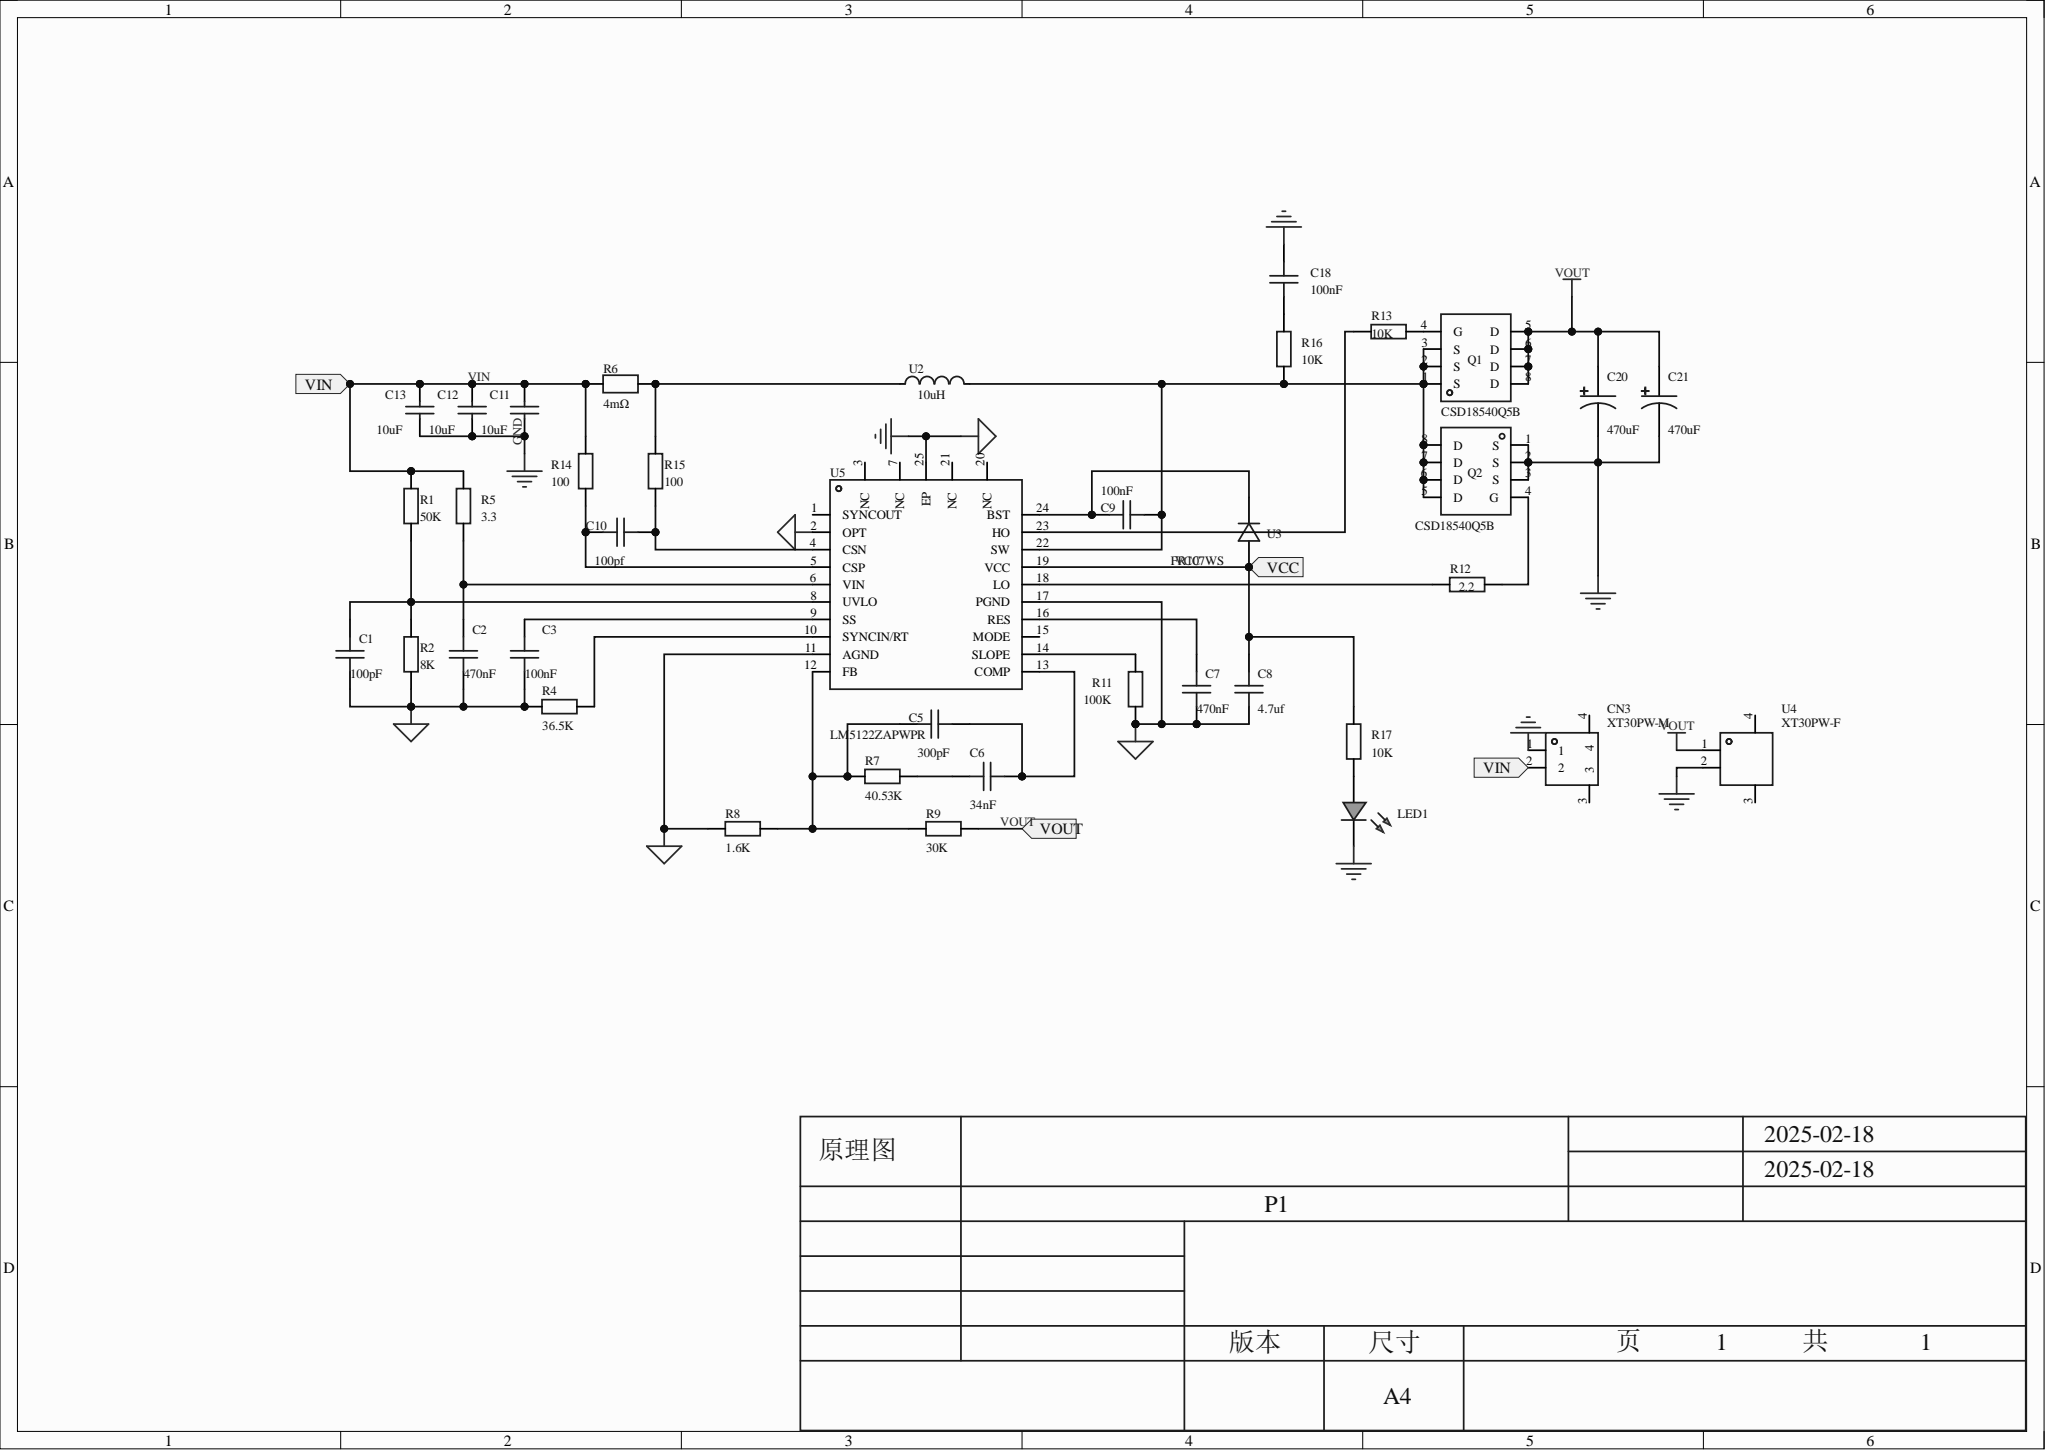Circuit board | Altium Designer | 38 parts | 24 nets
Bill of materials:
Comment,Description,Designator,Footprint,LibRef,Quantity
"100pF","","C1, C10","C0603","CAP_0603","2"
"470nF","","C2, C7","C0603","CAP_0603","2"
"100nF","","C3, C9, C18","C0603","CAP_0603","3"
"300pF","","C5","C0603","CAP_0603","1"
"34nF","","C6","C0603","CAP_0603","1"
"4.7uf","","C8","C0805","CAP_0805","1"
"10uF","","C11, C12, C13","C1210","1210B106K500NT_C116808","3"
"470uF","","C20, C21","CAP-TH_BD16.0-P7.50-D1.2-FD","NXA 100VB470 M 16*25","2"
"XT30PW-M","","CN3","CONN-TH_XT30PW-M","XT30PW-M","1"
"","","LED1","LED_0805","LED_0805-G","1"
"CSD18540Q5B","","Q1, Q2","VSON-CLIP-8_L5.0-W6.0-P1.27-BL","CSD18540Q5B","2"
"50K","","R1","R0603","Res_0603","1"
"8K","","R2","R0603","Res_0603","1"
"36.5K","","R4","R0603","Res_0603","1"
"3.3","","R5","R0805_NEW","Res_0603","1"
"4mΩ","","R6","RES-SMD_L6.4-W3.2-1","PA2512FKF7W0R05E","1"
"40.53K","","R7","R0603","Res_0603","1"
"1.6K","","R8","R0603","Res_0603","1"
"30K","","R9","R0603","Res_0603","1"
"100K","","R11","R0603","Res_0603","1"
"2.2","","R12","R0603","Res_0603","1"
"10K","","R13, R16","R0603","Res_0603","2"
"100","","R14, R15","R0603","Res_0603","2"
"10K","","R17","R0805","Res_0805","1"
"10uH","","U2","IND-SMD_L17.0-W17.0_YSPIA1770-100M","CY1770AT125DS-4R7MC","1"
"FR107WS","","U3","SOD-323_L1.6-W1.3-LS2.7-RD","FR107WS","1"
"XT30PW-F","","U4","CONN-TH_XT30PW-F-1","XT30PW-F","1"
"LM5122ZAPWPR","","U5","HTSSOP-24_L7.8-W4.4-P0.65-LS6.4-BL-EP-3","LM5122ZAPWPR","1"
Netlist (Protel format):
[
C1
C0603
100pF



]
[
C2
C0603
470nF



]
[
C3
C0603
100nF



]
[
C5
C0603
300pF



]
[
C6
C0603
34nF



]
[
C7
C0603
470nF



]
[
C8
C0805
4.7uf



]
[
C9
C0603
100nF



]
[
C10
C0603
100pf



]
[
C11
C1210
10uF



]
[
C12
C1210
10uF



]
[
C13
C1210
10uF



]
[
C18
C0603
100nF



]
[
C20
CAP-TH_BD16.0-P7.50-D1.2-FD
470uF



]
[
C21
CAP-TH_BD16.0-P7.50-D1.2-FD
470uF



]
[
CN3
CONN-TH_XT30PW-M
XT30PW-M



]
[
LED1
LED_0805




]
[
Q1
VSON-CLIP-8_L5.0-W6.0-P1.27-BL
CSD18540Q5B



]
[
Q2
VSON-CLIP-8_L5.0-W6.0-P1.27-BL
CSD18540Q5B



]
[
R1
R0603
50K



]
[
R2
R0603
8K



]
[
R4
R0603
36.5K



]
[
R5
R0805_NEW
3.3



]
[
R6
RES-SMD_L6.4-W3.2-1
4mΩ



]
[
R7
R0603
40.53K



]
[
R8
R0603
1.6K



]
[
R9
R0603
30K



]
[
R11
R0603
100K



]
[
R12
R0603
2.2



]
[
R13
R0603
10K



]
[
R14
R0603
100



]
[
R15
R0603
100



]
[
R16
R0603
10K



]
[
R17
R0805
10K



]
[
U2
IND-SMD_L17.0-W17.0_YSPIA1770-100M
10uH



]
[
U3
SOD-323_L1.6-W1.3-LS2.7-RD
FR107WS



]
[
U4
CONN-TH_XT30PW-F-1
XT30PW-F



]
[
U5
HTSSOP-24_L7.8-W4.4-P0.65-LS6.4-BL-EP-3
LM5122ZAPWPR



]
(
VOUT
C20-1
C21-1
Q1-5
Q1-6
Q1-7
Q1-8
R9-2
U4-1
)
(
VIN
C11-2
C12-2
C13-2
CN3-2
R1-2
R5-2
R6-1
R14-2
)
(
VCC
C8-1
R17-2
U3-2
U5-19
)
(
NetR13_1
R13-1
U5-23
)
(
NetR12_1
R12-1
U5-18
)
(
NetR11_2
R11-2
U5-14
)
(
NetR6_2
R6-2
R15-2
U2-1
)
(
NetR4_2
R4-2
U5-10
)
(
NetQ2_4
Q2-4
R12-2
)
(
NetQ1_4
Q1-4
R13-2
)
(
NetLED1_2
LED1-2
R17-1
)
(
NetC18_1
C18-1
R16-2
)
(
NetC10_2
C10-2
R15-1
U5-4
)
(
NetC10_1
C10-1
R14-1
U5-5
)
(
NetC9_2
C9-2
U3-1
U5-24
)
(
NetC9_1
C9-1
Q1-1
Q1-2
Q1-3
Q2-5
Q2-6
Q2-7
Q2-8
R16-1
U2-2
U5-22
)
(
NetC7_1
C7-1
U5-16
)
(
NetC6_1
C6-1
R7-2
)
(
NetC5_2
C5-2
C6-2
U5-13
)
(
NetC5_1
C5-1
R7-1
R8-2
R9-1
U5-12
)
(
NetC3_2
C3-2
U5-9
)
(
NetC2_2
C2-2
R5-1
U5-6
)
(
NetC1_2
C1-2
R1-1
R2-2
U5-8
)
(
GND
C1-1
C2-1
C3-1
C7-2
C8-2
C11-1
C12-1
C13-1
C18-2
C20-2
C21-2
CN3-1
LED1-1
Q2-1
Q2-2
Q2-3
R2-1
R4-1
R8-1
R11-1
U4-2
U5-2
U5-11
U5-17
U5-25
)